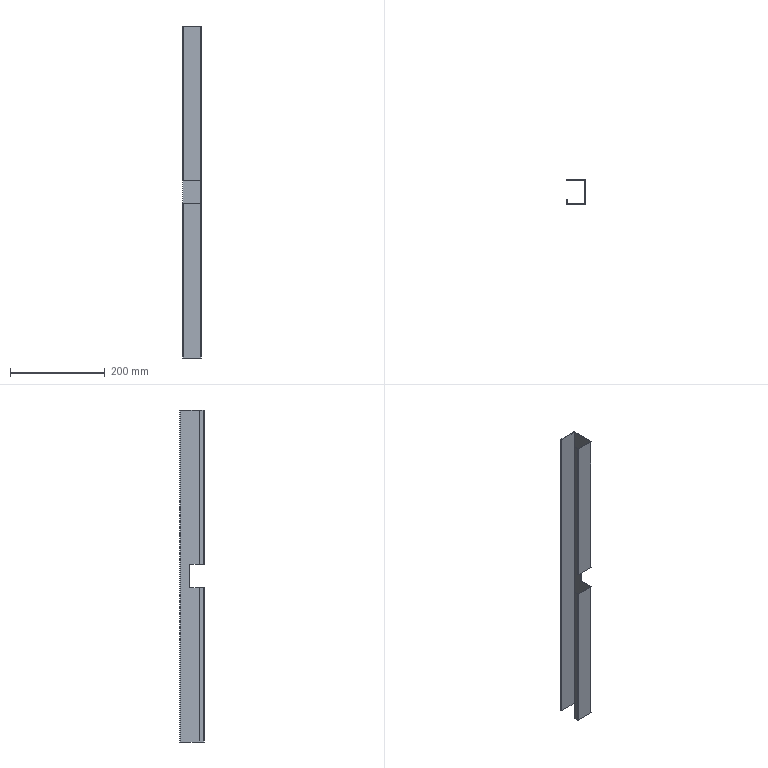Part | SolidWorks | features FlatPattern 1, ICE 1, SMBaseFlange 1, SheetMetal 1 | 1 solid | 50 faces | box 40 x 51 x 700 mm | volume 136327 mm3 | plane 40 | cylinder 10 | commonest cylinder face diameters 0.4 x5 3.4 x5
STEP:
#1=CARTESIAN_POINT('',(-20.,-41.,-25.));
#2=VERTEX_POINT('',#1);
#3=CARTESIAN_POINT('',(-20.,-49.3,-25.));
#4=VERTEX_POINT('',#3);
#5=CARTESIAN_POINT('',(-20.,-51.,-25.));
#6=DIRECTION('',(0.,-1.,0.));
#7=VECTOR('',#6,1000.);
#8=LINE('',#5,#7);
#9=EDGE_CURVE('',#2,#4,#8,.T.);
#10=ORIENTED_EDGE('',*,*,#9,.T.);
#11=CARTESIAN_POINT('',(-18.5,-49.3,-25.));
#12=VERTEX_POINT('',#11);
#13=CARTESIAN_POINT('',(-20.,-49.3,-25.));
#14=DIRECTION('',(1.,0.,0.));
#15=VECTOR('',#14,1000.);
#16=LINE('',#13,#15);
#17=EDGE_CURVE('',#4,#12,#16,.T.);
#18=ORIENTED_EDGE('',*,*,#17,.T.);
#19=CARTESIAN_POINT('',(-18.5,-41.,-25.));
#20=VERTEX_POINT('',#19);
#21=CARTESIAN_POINT('',(-18.5,-51.,-25.));
#22=DIRECTION('',(0.,-1.,0.));
#23=VECTOR('',#22,1000.);
#24=LINE('',#21,#23);
#25=EDGE_CURVE('',#20,#12,#24,.T.);
#26=ORIENTED_EDGE('',*,*,#25,.F.);
#27=CARTESIAN_POINT('',(-20.,-41.,-25.));
#28=DIRECTION('',(-1.,0.,0.));
#29=VECTOR('',#28,1000.);
#30=LINE('',#27,#29);
#31=EDGE_CURVE('',#20,#2,#30,.T.);
#32=ORIENTED_EDGE('',*,*,#31,.T.);
#33=EDGE_LOOP('',(#10,#18,#26,#32));
#34=FACE_OUTER_BOUND('',#33,.T.);
#35=CARTESIAN_POINT('',(40.,-21.,-25.));
#36=DIRECTION('',(0.,0.,-1.));
#37=DIRECTION('',(-1.,0.,0.));
#38=AXIS2_PLACEMENT_3D('',#35,#36,#37);
#39=PLANE('',#38);
#40=ADVANCED_FACE('',(#34),#39,.F.);
#41=CARTESIAN_POINT('',(-18.3,-49.5,-25.));
#42=VERTEX_POINT('',#41);
#43=CARTESIAN_POINT('',(18.3,-49.5,-25.));
#44=VERTEX_POINT('',#43);
#45=CARTESIAN_POINT('',(20.,-49.5,-25.));
#46=DIRECTION('',(1.,0.,0.));
#47=VECTOR('',#46,1000.);
#48=LINE('',#45,#47);
#49=EDGE_CURVE('',#42,#44,#48,.T.);
#50=ORIENTED_EDGE('',*,*,#49,.F.);
#51=CARTESIAN_POINT('',(-18.3,-51.,-25.));
#52=VERTEX_POINT('',#51);
#53=CARTESIAN_POINT('',(-18.3,-49.5,-25.));
#54=DIRECTION('',(0.,-1.,0.));
#55=VECTOR('',#54,1000.);
#56=LINE('',#53,#55);
#57=EDGE_CURVE('',#42,#52,#56,.T.);
#58=ORIENTED_EDGE('',*,*,#57,.T.);
#59=CARTESIAN_POINT('',(18.3,-51.,-25.));
#60=VERTEX_POINT('',#59);
#61=CARTESIAN_POINT('',(40.,-51.,-25.));
#62=DIRECTION('',(1.,0.,0.));
#63=VECTOR('',#62,1000.);
#64=LINE('',#61,#63);
#65=EDGE_CURVE('',#52,#60,#64,.T.);
#66=ORIENTED_EDGE('',*,*,#65,.T.);
#67=CARTESIAN_POINT('',(18.3,-51.,-25.));
#68=DIRECTION('',(0.,1.,0.));
#69=VECTOR('',#68,1000.);
#70=LINE('',#67,#69);
#71=EDGE_CURVE('',#60,#44,#70,.T.);
#72=ORIENTED_EDGE('',*,*,#71,.T.);
#73=EDGE_LOOP('',(#50,#58,#66,#72));
#74=FACE_OUTER_BOUND('',#73,.T.);
#75=CARTESIAN_POINT('',(40.,-21.,-25.));
#76=DIRECTION('',(0.,0.,-1.));
#77=DIRECTION('',(-1.,0.,0.));
#78=AXIS2_PLACEMENT_3D('',#75,#76,#77);
#79=PLANE('',#78);
#80=ADVANCED_FACE('',(#74),#79,.F.);
#81=CARTESIAN_POINT('',(18.5,-49.3,-25.));
#82=VERTEX_POINT('',#81);
#83=CARTESIAN_POINT('',(18.5,-21.,-25.));
#84=VERTEX_POINT('',#83);
#85=CARTESIAN_POINT('',(18.5,0.,-25.));
#86=DIRECTION('',(0.,1.,0.));
#87=VECTOR('',#86,1000.);
#88=LINE('',#85,#87);
#89=EDGE_CURVE('',#82,#84,#88,.T.);
#90=ORIENTED_EDGE('',*,*,#89,.F.);
#91=CARTESIAN_POINT('',(20.,-49.3,-25.));
#92=VERTEX_POINT('',#91);
#93=CARTESIAN_POINT('',(18.5,-49.3,-25.));
#94=DIRECTION('',(1.,0.,0.));
#95=VECTOR('',#94,1000.);
#96=LINE('',#93,#95);
#97=EDGE_CURVE('',#82,#92,#96,.T.);
#98=ORIENTED_EDGE('',*,*,#97,.T.);
#99=CARTESIAN_POINT('',(20.,-21.,-25.));
#100=VERTEX_POINT('',#99);
#101=CARTESIAN_POINT('',(20.,0.,-25.));
#102=DIRECTION('',(0.,1.,0.));
#103=VECTOR('',#102,1000.);
#104=LINE('',#101,#103);
#105=EDGE_CURVE('',#92,#100,#104,.T.);
#106=ORIENTED_EDGE('',*,*,#105,.T.);
#107=CARTESIAN_POINT('',(40.,-21.,-25.));
#108=DIRECTION('',(1.,0.,0.));
#109=VECTOR('',#108,1000.);
#110=LINE('',#107,#109);
#111=EDGE_CURVE('',#84,#100,#110,.T.);
#112=ORIENTED_EDGE('',*,*,#111,.F.);
#113=EDGE_LOOP('',(#90,#98,#106,#112));
#114=FACE_OUTER_BOUND('',#113,.T.);
#115=CARTESIAN_POINT('',(40.,-21.,-25.));
#116=DIRECTION('',(0.,0.,-1.));
#117=DIRECTION('',(-1.,0.,0.));
#118=AXIS2_PLACEMENT_3D('',#115,#116,#117);
#119=PLANE('',#118);
#120=ADVANCED_FACE('',(#114),#119,.F.);
#121=ORIENTED_EDGE('',*,*,#17,.F.);
#122=CARTESIAN_POINT('',(-18.3,-49.3,-25.));
#123=DIRECTION('',(0.,0.,1.));
#124=DIRECTION('',(-1.,0.,0.));
#125=AXIS2_PLACEMENT_3D('',#122,#123,#124);
#126=CIRCLE('',#125,1.7);
#127=EDGE_CURVE('',#4,#52,#126,.T.);
#128=ORIENTED_EDGE('',*,*,#127,.T.);
#129=ORIENTED_EDGE('',*,*,#57,.F.);
#130=CARTESIAN_POINT('',(-18.3,-49.3,-25.));
#131=DIRECTION('',(0.,0.,1.));
#132=DIRECTION('',(-1.,0.,0.));
#133=AXIS2_PLACEMENT_3D('',#130,#131,#132);
#134=CIRCLE('',#133,0.2);
#135=EDGE_CURVE('',#12,#42,#134,.T.);
#136=ORIENTED_EDGE('',*,*,#135,.F.);
#137=EDGE_LOOP('',(#121,#128,#129,#136));
#138=FACE_OUTER_BOUND('',#137,.T.);
#139=CARTESIAN_POINT('',(40.,-21.,-25.));
#140=DIRECTION('',(0.,0.,-1.));
#141=DIRECTION('',(-1.,0.,0.));
#142=AXIS2_PLACEMENT_3D('',#139,#140,#141);
#143=PLANE('',#142);
#144=ADVANCED_FACE('',(#138),#143,.F.);
#145=CARTESIAN_POINT('',(-18.5,-49.3,25.));
#146=VERTEX_POINT('',#145);
#147=CARTESIAN_POINT('',(-18.5,-41.,25.));
#148=VERTEX_POINT('',#147);
#149=CARTESIAN_POINT('',(-18.5,-51.,25.));
#150=DIRECTION('',(0.,1.,0.));
#151=VECTOR('',#150,1000.);
#152=LINE('',#149,#151);
#153=EDGE_CURVE('',#146,#148,#152,.T.);
#154=ORIENTED_EDGE('',*,*,#153,.F.);
#155=CARTESIAN_POINT('',(-20.,-49.3,25.));
#156=VERTEX_POINT('',#155);
#157=CARTESIAN_POINT('',(-18.5,-49.3,25.));
#158=DIRECTION('',(-1.,0.,0.));
#159=VECTOR('',#158,1000.);
#160=LINE('',#157,#159);
#161=EDGE_CURVE('',#146,#156,#160,.T.);
#162=ORIENTED_EDGE('',*,*,#161,.T.);
#163=CARTESIAN_POINT('',(-20.,-41.,25.));
#164=VERTEX_POINT('',#163);
#165=CARTESIAN_POINT('',(-20.,-51.,25.));
#166=DIRECTION('',(0.,1.,0.));
#167=VECTOR('',#166,1000.);
#168=LINE('',#165,#167);
#169=EDGE_CURVE('',#156,#164,#168,.T.);
#170=ORIENTED_EDGE('',*,*,#169,.T.);
#171=CARTESIAN_POINT('',(-20.,-41.,25.));
#172=DIRECTION('',(1.,0.,0.));
#173=VECTOR('',#172,1000.);
#174=LINE('',#171,#173);
#175=EDGE_CURVE('',#164,#148,#174,.T.);
#176=ORIENTED_EDGE('',*,*,#175,.T.);
#177=EDGE_LOOP('',(#154,#162,#170,#176));
#178=FACE_OUTER_BOUND('',#177,.T.);
#179=CARTESIAN_POINT('',(40.,-21.,25.));
#180=DIRECTION('',(0.,0.,1.));
#181=DIRECTION('',(1.,0.,0.));
#182=AXIS2_PLACEMENT_3D('',#179,#180,#181);
#183=PLANE('',#182);
#184=ADVANCED_FACE('',(#178),#183,.F.);
#185=CARTESIAN_POINT('',(18.3,-51.,25.));
#186=VERTEX_POINT('',#185);
#187=CARTESIAN_POINT('',(-18.3,-51.,25.));
#188=VERTEX_POINT('',#187);
#189=CARTESIAN_POINT('',(40.,-51.,25.));
#190=DIRECTION('',(-1.,0.,0.));
#191=VECTOR('',#190,1000.);
#192=LINE('',#189,#191);
#193=EDGE_CURVE('',#186,#188,#192,.T.);
#194=ORIENTED_EDGE('',*,*,#193,.T.);
#195=CARTESIAN_POINT('',(-18.3,-49.5,25.));
#196=VERTEX_POINT('',#195);
#197=CARTESIAN_POINT('',(-18.3,-51.,25.));
#198=DIRECTION('',(0.,1.,0.));
#199=VECTOR('',#198,1000.);
#200=LINE('',#197,#199);
#201=EDGE_CURVE('',#188,#196,#200,.T.);
#202=ORIENTED_EDGE('',*,*,#201,.T.);
#203=CARTESIAN_POINT('',(18.3,-49.5,25.));
#204=VERTEX_POINT('',#203);
#205=CARTESIAN_POINT('',(20.,-49.5,25.));
#206=DIRECTION('',(-1.,0.,0.));
#207=VECTOR('',#206,1000.);
#208=LINE('',#205,#207);
#209=EDGE_CURVE('',#204,#196,#208,.T.);
#210=ORIENTED_EDGE('',*,*,#209,.F.);
#211=CARTESIAN_POINT('',(18.3,-49.5,25.));
#212=DIRECTION('',(0.,-1.,0.));
#213=VECTOR('',#212,1000.);
#214=LINE('',#211,#213);
#215=EDGE_CURVE('',#204,#186,#214,.T.);
#216=ORIENTED_EDGE('',*,*,#215,.T.);
#217=EDGE_LOOP('',(#194,#202,#210,#216));
#218=FACE_OUTER_BOUND('',#217,.T.);
#219=CARTESIAN_POINT('',(40.,-21.,25.));
#220=DIRECTION('',(0.,0.,1.));
#221=DIRECTION('',(1.,0.,0.));
#222=AXIS2_PLACEMENT_3D('',#219,#220,#221);
#223=PLANE('',#222);
#224=ADVANCED_FACE('',(#218),#223,.F.);
#225=ORIENTED_EDGE('',*,*,#161,.F.);
#226=CARTESIAN_POINT('',(-18.3,-49.3,25.));
#227=DIRECTION('',(0.,0.,-1.));
#228=DIRECTION('',(1.,0.,0.));
#229=AXIS2_PLACEMENT_3D('',#226,#227,#228);
#230=CIRCLE('',#229,0.2);
#231=EDGE_CURVE('',#196,#146,#230,.T.);
#232=ORIENTED_EDGE('',*,*,#231,.F.);
#233=ORIENTED_EDGE('',*,*,#201,.F.);
#234=CARTESIAN_POINT('',(-18.3,-49.3,25.));
#235=DIRECTION('',(0.,0.,-1.));
#236=DIRECTION('',(1.,0.,0.));
#237=AXIS2_PLACEMENT_3D('',#234,#235,#236);
#238=CIRCLE('',#237,1.7);
#239=EDGE_CURVE('',#188,#156,#238,.T.);
#240=ORIENTED_EDGE('',*,*,#239,.T.);
#241=EDGE_LOOP('',(#225,#232,#233,#240));
#242=FACE_OUTER_BOUND('',#241,.T.);
#243=CARTESIAN_POINT('',(40.,-21.,25.));
#244=DIRECTION('',(0.,0.,1.));
#245=DIRECTION('',(1.,0.,0.));
#246=AXIS2_PLACEMENT_3D('',#243,#244,#245);
#247=PLANE('',#246);
#248=ADVANCED_FACE('',(#242),#247,.F.);
#249=CARTESIAN_POINT('',(20.,-21.,25.));
#250=VERTEX_POINT('',#249);
#251=CARTESIAN_POINT('',(20.,-49.3,25.));
#252=VERTEX_POINT('',#251);
#253=CARTESIAN_POINT('',(20.,0.,25.));
#254=DIRECTION('',(0.,-1.,0.));
#255=VECTOR('',#254,1000.);
#256=LINE('',#253,#255);
#257=EDGE_CURVE('',#250,#252,#256,.T.);
#258=ORIENTED_EDGE('',*,*,#257,.T.);
#259=CARTESIAN_POINT('',(18.5,-49.3,25.));
#260=VERTEX_POINT('',#259);
#261=CARTESIAN_POINT('',(20.,-49.3,25.));
#262=DIRECTION('',(-1.,0.,0.));
#263=VECTOR('',#262,1000.);
#264=LINE('',#261,#263);
#265=EDGE_CURVE('',#252,#260,#264,.T.);
#266=ORIENTED_EDGE('',*,*,#265,.T.);
#267=CARTESIAN_POINT('',(18.5,-21.,25.));
#268=VERTEX_POINT('',#267);
#269=CARTESIAN_POINT('',(18.5,0.,25.));
#270=DIRECTION('',(0.,-1.,0.));
#271=VECTOR('',#270,1000.);
#272=LINE('',#269,#271);
#273=EDGE_CURVE('',#268,#260,#272,.T.);
#274=ORIENTED_EDGE('',*,*,#273,.F.);
#275=CARTESIAN_POINT('',(40.,-21.,25.));
#276=DIRECTION('',(-1.,0.,0.));
#277=VECTOR('',#276,1000.);
#278=LINE('',#275,#277);
#279=EDGE_CURVE('',#250,#268,#278,.T.);
#280=ORIENTED_EDGE('',*,*,#279,.F.);
#281=EDGE_LOOP('',(#258,#266,#274,#280));
#282=FACE_OUTER_BOUND('',#281,.T.);
#283=CARTESIAN_POINT('',(40.,-21.,25.));
#284=DIRECTION('',(0.,0.,1.));
#285=DIRECTION('',(1.,0.,0.));
#286=AXIS2_PLACEMENT_3D('',#283,#284,#285);
#287=PLANE('',#286);
#288=ADVANCED_FACE('',(#282),#287,.F.);
#289=CARTESIAN_POINT('',(-18.5,-49.3,350.));
#290=VERTEX_POINT('',#289);
#291=CARTESIAN_POINT('',(-18.5,-49.3,350.));
#292=DIRECTION('',(0.,0.,-1.));
#293=VECTOR('',#292,1000.);
#294=LINE('',#291,#293);
#295=EDGE_CURVE('',#290,#146,#294,.T.);
#296=ORIENTED_EDGE('',*,*,#295,.T.);
#297=ORIENTED_EDGE('',*,*,#153,.T.);
#298=CARTESIAN_POINT('',(-18.5,-41.,350.));
#299=VERTEX_POINT('',#298);
#300=CARTESIAN_POINT('',(-18.5,-41.,350.));
#301=DIRECTION('',(0.,0.,-1.));
#302=VECTOR('',#301,1000.);
#303=LINE('',#300,#302);
#304=EDGE_CURVE('',#299,#148,#303,.T.);
#305=ORIENTED_EDGE('',*,*,#304,.F.);
#306=CARTESIAN_POINT('',(-18.5,-51.,350.));
#307=DIRECTION('',(0.,1.,0.));
#308=VECTOR('',#307,1000.);
#309=LINE('',#306,#308);
#310=EDGE_CURVE('',#290,#299,#309,.T.);
#311=ORIENTED_EDGE('',*,*,#310,.F.);
#312=EDGE_LOOP('',(#296,#297,#305,#311));
#313=FACE_OUTER_BOUND('',#312,.T.);
#314=CARTESIAN_POINT('',(-18.5,-51.,350.));
#315=DIRECTION('',(-1.,0.,0.));
#316=DIRECTION('',(0.,-1.,0.));
#317=AXIS2_PLACEMENT_3D('',#314,#315,#316);
#318=PLANE('',#317);
#319=ADVANCED_FACE('',(#313),#318,.F.);
#320=ORIENTED_EDGE('',*,*,#175,.F.);
#321=CARTESIAN_POINT('',(-20.,-41.,350.));
#322=VERTEX_POINT('',#321);
#323=CARTESIAN_POINT('',(-20.,-41.,350.));
#324=DIRECTION('',(0.,0.,-1.));
#325=VECTOR('',#324,1000.);
#326=LINE('',#323,#325);
#327=EDGE_CURVE('',#322,#164,#326,.T.);
#328=ORIENTED_EDGE('',*,*,#327,.F.);
#329=CARTESIAN_POINT('',(-20.,-41.,350.));
#330=DIRECTION('',(1.,0.,0.));
#331=VECTOR('',#330,1000.);
#332=LINE('',#329,#331);
#333=EDGE_CURVE('',#322,#299,#332,.T.);
#334=ORIENTED_EDGE('',*,*,#333,.T.);
#335=ORIENTED_EDGE('',*,*,#304,.T.);
#336=EDGE_LOOP('',(#320,#328,#334,#335));
#337=FACE_OUTER_BOUND('',#336,.T.);
#338=CARTESIAN_POINT('',(-20.,-41.,350.));
#339=DIRECTION('',(0.,1.,0.));
#340=DIRECTION('',(0.,0.,1.));
#341=AXIS2_PLACEMENT_3D('',#338,#339,#340);
#342=PLANE('',#341);
#343=ADVANCED_FACE('',(#337),#342,.T.);
#344=ORIENTED_EDGE('',*,*,#169,.F.);
#345=CARTESIAN_POINT('',(-20.,-49.3,350.));
#346=VERTEX_POINT('',#345);
#347=CARTESIAN_POINT('',(-20.,-49.3,350.));
#348=DIRECTION('',(0.,0.,-1.));
#349=VECTOR('',#348,1000.);
#350=LINE('',#347,#349);
#351=EDGE_CURVE('',#346,#156,#350,.T.);
#352=ORIENTED_EDGE('',*,*,#351,.F.);
#353=CARTESIAN_POINT('',(-20.,-51.,350.));
#354=DIRECTION('',(0.,1.,0.));
#355=VECTOR('',#354,1000.);
#356=LINE('',#353,#355);
#357=EDGE_CURVE('',#346,#322,#356,.T.);
#358=ORIENTED_EDGE('',*,*,#357,.T.);
#359=ORIENTED_EDGE('',*,*,#327,.T.);
#360=EDGE_LOOP('',(#344,#352,#358,#359));
#361=FACE_OUTER_BOUND('',#360,.T.);
#362=CARTESIAN_POINT('',(-20.,-51.,350.));
#363=DIRECTION('',(-1.,0.,0.));
#364=DIRECTION('',(0.,-1.,0.));
#365=AXIS2_PLACEMENT_3D('',#362,#363,#364);
#366=PLANE('',#365);
#367=ADVANCED_FACE('',(#361),#366,.T.);
#368=ORIENTED_EDGE('',*,*,#239,.F.);
#369=CARTESIAN_POINT('',(-18.3,-51.,350.));
#370=VERTEX_POINT('',#369);
#371=CARTESIAN_POINT('',(-18.3,-51.,350.));
#372=DIRECTION('',(0.,0.,-1.));
#373=VECTOR('',#372,1000.);
#374=LINE('',#371,#373);
#375=EDGE_CURVE('',#370,#188,#374,.T.);
#376=ORIENTED_EDGE('',*,*,#375,.F.);
#377=CARTESIAN_POINT('',(-18.3,-49.3,350.));
#378=DIRECTION('',(0.,0.,-1.));
#379=DIRECTION('',(1.,0.,0.));
#380=AXIS2_PLACEMENT_3D('',#377,#378,#379);
#381=CIRCLE('',#380,1.7);
#382=EDGE_CURVE('',#370,#346,#381,.T.);
#383=ORIENTED_EDGE('',*,*,#382,.T.);
#384=ORIENTED_EDGE('',*,*,#351,.T.);
#385=EDGE_LOOP('',(#368,#376,#383,#384));
#386=FACE_OUTER_BOUND('',#385,.T.);
#387=CARTESIAN_POINT('',(-18.3,-49.3,350.));
#388=DIRECTION('',(0.,0.,-1.));
#389=DIRECTION('',(-1.,0.,0.));
#390=AXIS2_PLACEMENT_3D('',#387,#388,#389);
#391=CYLINDRICAL_SURFACE('',#390,1.7);
#392=ADVANCED_FACE('',(#386),#391,.T.);
#393=ORIENTED_EDGE('',*,*,#193,.F.);
#394=CARTESIAN_POINT('',(18.3,-51.,350.));
#395=VERTEX_POINT('',#394);
#396=CARTESIAN_POINT('',(18.3,-51.,350.));
#397=DIRECTION('',(0.,0.,-1.));
#398=VECTOR('',#397,1000.);
#399=LINE('',#396,#398);
#400=EDGE_CURVE('',#395,#186,#399,.T.);
#401=ORIENTED_EDGE('',*,*,#400,.F.);
#402=CARTESIAN_POINT('',(20.,-51.,350.));
#403=DIRECTION('',(-1.,0.,0.));
#404=VECTOR('',#403,1000.);
#405=LINE('',#402,#404);
#406=EDGE_CURVE('',#395,#370,#405,.T.);
#407=ORIENTED_EDGE('',*,*,#406,.T.);
#408=ORIENTED_EDGE('',*,*,#375,.T.);
#409=EDGE_LOOP('',(#393,#401,#407,#408));
#410=FACE_OUTER_BOUND('',#409,.T.);
#411=CARTESIAN_POINT('',(20.,-51.,350.));
#412=DIRECTION('',(0.,-1.,0.));
#413=DIRECTION('',(1.,0.,0.));
#414=AXIS2_PLACEMENT_3D('',#411,#412,#413);
#415=PLANE('',#414);
#416=ADVANCED_FACE('',(#410),#415,.T.);
#417=CARTESIAN_POINT('',(18.3,-49.3,25.));
#418=DIRECTION('',(0.,0.,-1.));
#419=DIRECTION('',(1.,0.,0.));
#420=AXIS2_PLACEMENT_3D('',#417,#418,#419);
#421=CIRCLE('',#420,1.7);
#422=EDGE_CURVE('',#252,#186,#421,.T.);
#423=ORIENTED_EDGE('',*,*,#422,.F.);
#424=CARTESIAN_POINT('',(20.,-49.3,350.));
#425=VERTEX_POINT('',#424);
#426=CARTESIAN_POINT('',(20.,-49.3,350.));
#427=DIRECTION('',(0.,0.,-1.));
#428=VECTOR('',#427,1000.);
#429=LINE('',#426,#428);
#430=EDGE_CURVE('',#425,#252,#429,.T.);
#431=ORIENTED_EDGE('',*,*,#430,.F.);
#432=CARTESIAN_POINT('',(18.3,-49.3,350.));
#433=DIRECTION('',(0.,0.,-1.));
#434=DIRECTION('',(1.,0.,0.));
#435=AXIS2_PLACEMENT_3D('',#432,#433,#434);
#436=CIRCLE('',#435,1.7);
#437=EDGE_CURVE('',#425,#395,#436,.T.);
#438=ORIENTED_EDGE('',*,*,#437,.T.);
#439=ORIENTED_EDGE('',*,*,#400,.T.);
#440=EDGE_LOOP('',(#423,#431,#438,#439));
#441=FACE_OUTER_BOUND('',#440,.T.);
#442=CARTESIAN_POINT('',(18.3,-49.3,350.));
#443=DIRECTION('',(0.,0.,-1.));
#444=DIRECTION('',(-1.,0.,0.));
#445=AXIS2_PLACEMENT_3D('',#442,#443,#444);
#446=CYLINDRICAL_SURFACE('',#445,1.7);
#447=ADVANCED_FACE('',(#441),#446,.T.);
#448=CARTESIAN_POINT('',(18.5,-49.3,350.));
#449=VERTEX_POINT('',#448);
#450=CARTESIAN_POINT('',(18.5,-49.3,350.));
#451=DIRECTION('',(0.,0.,-1.));
#452=VECTOR('',#451,1000.);
#453=LINE('',#450,#452);
#454=EDGE_CURVE('',#449,#260,#453,.T.);
#455=ORIENTED_EDGE('',*,*,#454,.T.);
#456=CARTESIAN_POINT('',(18.3,-49.3,25.));
#457=DIRECTION('',(0.,0.,-1.));
#458=DIRECTION('',(1.,0.,0.));
#459=AXIS2_PLACEMENT_3D('',#456,#457,#458);
#460=CIRCLE('',#459,0.2);
#461=EDGE_CURVE('',#260,#204,#460,.T.);
#462=ORIENTED_EDGE('',*,*,#461,.T.);
#463=CARTESIAN_POINT('',(18.3,-49.5,350.));
#464=VERTEX_POINT('',#463);
#465=CARTESIAN_POINT('',(18.3,-49.5,350.));
#466=DIRECTION('',(0.,0.,-1.));
#467=VECTOR('',#466,1000.);
#468=LINE('',#465,#467);
#469=EDGE_CURVE('',#464,#204,#468,.T.);
#470=ORIENTED_EDGE('',*,*,#469,.F.);
#471=CARTESIAN_POINT('',(18.3,-49.3,350.));
#472=DIRECTION('',(0.,0.,-1.));
#473=DIRECTION('',(1.,0.,0.));
#474=AXIS2_PLACEMENT_3D('',#471,#472,#473);
#475=CIRCLE('',#474,0.2);
#476=EDGE_CURVE('',#449,#464,#475,.T.);
#477=ORIENTED_EDGE('',*,*,#476,.F.);
#478=EDGE_LOOP('',(#455,#462,#470,#477));
#479=FACE_OUTER_BOUND('',#478,.T.);
#480=CARTESIAN_POINT('',(18.3,-49.3,350.));
#481=DIRECTION('',(0.,0.,-1.));
#482=DIRECTION('',(-1.,0.,0.));
#483=AXIS2_PLACEMENT_3D('',#480,#481,#482);
#484=CYLINDRICAL_SURFACE('',#483,0.2);
#485=ADVANCED_FACE('',(#479),#484,.F.);
#486=ORIENTED_EDGE('',*,*,#469,.T.);
#487=ORIENTED_EDGE('',*,*,#209,.T.);
#488=CARTESIAN_POINT('',(-18.3,-49.5,350.));
#489=VERTEX_POINT('',#488);
#490=CARTESIAN_POINT('',(-18.3,-49.5,350.));
#491=DIRECTION('',(0.,0.,-1.));
#492=VECTOR('',#491,1000.);
#493=LINE('',#490,#492);
#494=EDGE_CURVE('',#489,#196,#493,.T.);
#495=ORIENTED_EDGE('',*,*,#494,.F.);
#496=CARTESIAN_POINT('',(20.,-49.5,350.));
#497=DIRECTION('',(-1.,0.,0.));
#498=VECTOR('',#497,1000.);
#499=LINE('',#496,#498);
#500=EDGE_CURVE('',#464,#489,#499,.T.);
#501=ORIENTED_EDGE('',*,*,#500,.F.);
#502=EDGE_LOOP('',(#486,#487,#495,#501));
#503=FACE_OUTER_BOUND('',#502,.T.);
#504=CARTESIAN_POINT('',(20.,-49.5,350.));
#505=DIRECTION('',(0.,-1.,0.));
#506=DIRECTION('',(1.,0.,0.));
#507=AXIS2_PLACEMENT_3D('',#504,#505,#506);
#508=PLANE('',#507);
#509=ADVANCED_FACE('',(#503),#508,.F.);
#510=ORIENTED_EDGE('',*,*,#494,.T.);
#511=ORIENTED_EDGE('',*,*,#231,.T.);
#512=ORIENTED_EDGE('',*,*,#295,.F.);
#513=CARTESIAN_POINT('',(-18.3,-49.3,350.));
#514=DIRECTION('',(0.,0.,-1.));
#515=DIRECTION('',(1.,0.,0.));
#516=AXIS2_PLACEMENT_3D('',#513,#514,#515);
#517=CIRCLE('',#516,0.2);
#518=EDGE_CURVE('',#489,#290,#517,.T.);
#519=ORIENTED_EDGE('',*,*,#518,.F.);
#520=EDGE_LOOP('',(#510,#511,#512,#519));
#521=FACE_OUTER_BOUND('',#520,.T.);
#522=CARTESIAN_POINT('',(-18.3,-49.3,350.));
#523=DIRECTION('',(0.,0.,-1.));
#524=DIRECTION('',(-1.,0.,0.));
#525=AXIS2_PLACEMENT_3D('',#522,#523,#524);
#526=CYLINDRICAL_SURFACE('',#525,0.2);
#527=ADVANCED_FACE('',(#521),#526,.F.);
#528=CARTESIAN_POINT('',(20.,-1.7,350.));
#529=VERTEX_POINT('',#528);
#530=CARTESIAN_POINT('',(18.5,-1.7,350.));
#531=VERTEX_POINT('',#530);
#532=CARTESIAN_POINT('',(20.,-1.7,350.));
#533=DIRECTION('',(-1.,0.,0.));
#534=VECTOR('',#533,1000.);
#535=LINE('',#532,#534);
#536=EDGE_CURVE('',#529,#531,#535,.T.);
#537=ORIENTED_EDGE('',*,*,#536,.F.);
#538=CARTESIAN_POINT('',(18.3,0.,350.));
#539=VERTEX_POINT('',#538);
#540=CARTESIAN_POINT('',(18.3,-1.7,350.));
#541=DIRECTION('',(0.,0.,-1.));
#542=DIRECTION('',(1.,0.,0.));
#543=AXIS2_PLACEMENT_3D('',#540,#541,#542);
#544=CIRCLE('',#543,1.7);
#545=EDGE_CURVE('',#539,#529,#544,.T.);
#546=ORIENTED_EDGE('',*,*,#545,.F.);
#547=CARTESIAN_POINT('',(18.3,-1.5,350.));
#548=VERTEX_POINT('',#547);
#549=CARTESIAN_POINT('',(18.3,-1.5,350.));
#550=DIRECTION('',(0.,1.,0.));
#551=VECTOR('',#550,1000.);
#552=LINE('',#549,#551);
#553=EDGE_CURVE('',#548,#539,#552,.T.);
#554=ORIENTED_EDGE('',*,*,#553,.F.);
#555=CARTESIAN_POINT('',(18.3,-1.7,350.));
#556=DIRECTION('',(0.,0.,-1.));
#557=DIRECTION('',(1.,0.,0.));
#558=AXIS2_PLACEMENT_3D('',#555,#556,#557);
#559=CIRCLE('',#558,0.2);
#560=EDGE_CURVE('',#548,#531,#559,.T.);
#561=ORIENTED_EDGE('',*,*,#560,.T.);
#562=EDGE_LOOP('',(#537,#546,#554,#561));
#563=FACE_OUTER_BOUND('',#562,.T.);
#564=CARTESIAN_POINT('',(20.,-1.7,350.));
#565=DIRECTION('',(0.,0.,1.));
#566=DIRECTION('',(1.,0.,0.));
#567=AXIS2_PLACEMENT_3D('',#564,#565,#566);
#568=PLANE('',#567);
#569=ADVANCED_FACE('',(#563),#568,.T.);
#570=CARTESIAN_POINT('',(20.,0.,350.));
#571=DIRECTION('',(0.,-1.,0.));
#572=VECTOR('',#571,1000.);
#573=LINE('',#570,#572);
#574=EDGE_CURVE('',#529,#425,#573,.T.);
#575=ORIENTED_EDGE('',*,*,#574,.F.);
#576=ORIENTED_EDGE('',*,*,#536,.T.);
#577=CARTESIAN_POINT('',(18.5,0.,350.));
#578=DIRECTION('',(0.,-1.,0.));
#579=VECTOR('',#578,1000.);
#580=LINE('',#577,#579);
#581=EDGE_CURVE('',#531,#449,#580,.T.);
#582=ORIENTED_EDGE('',*,*,#581,.T.);
#583=CARTESIAN_POINT('',(18.5,-49.3,350.));
#584=DIRECTION('',(1.,0.,0.));
#585=VECTOR('',#584,1000.);
#586=LINE('',#583,#585);
#587=EDGE_CURVE('',#449,#425,#586,.T.);
#588=ORIENTED_EDGE('',*,*,#587,.T.);
#589=EDGE_LOOP('',(#575,#576,#582,#588));
#590=FACE_OUTER_BOUND('',#589,.T.);
#591=CARTESIAN_POINT('',(18.3,-1.5,350.));
#592=DIRECTION('',(0.,0.,1.));
#593=DIRECTION('',(1.,0.,0.));
#594=AXIS2_PLACEMENT_3D('',#591,#592,#593);
#595=PLANE('',#594);
#596=ADVANCED_FACE('',(#590),#595,.T.);
#597=CARTESIAN_POINT('',(18.3,0.,-350.));
#598=VERTEX_POINT('',#597);
#599=CARTESIAN_POINT('',(18.3,-1.5,-350.));
#600=VERTEX_POINT('',#599);
#601=CARTESIAN_POINT('',(18.3,0.,-350.));
#602=DIRECTION('',(0.,-1.,0.));
#603=VECTOR('',#602,1000.);
#604=LINE('',#601,#603);
#605=EDGE_CURVE('',#598,#600,#604,.T.);
#606=ORIENTED_EDGE('',*,*,#605,.F.);
#607=CARTESIAN_POINT('',(20.,-1.7,-350.));
#608=VERTEX_POINT('',#607);
#609=CARTESIAN_POINT('',(18.3,-1.7,-350.));
#610=DIRECTION('',(0.,0.,-1.));
#611=DIRECTION('',(1.,0.,0.));
#612=AXIS2_PLACEMENT_3D('',#609,#610,#611);
#613=CIRCLE('',#612,1.7);
#614=EDGE_CURVE('',#598,#608,#613,.T.);
#615=ORIENTED_EDGE('',*,*,#614,.T.);
#616=CARTESIAN_POINT('',(18.5,-1.7,-350.));
#617=VERTEX_POINT('',#616);
#618=CARTESIAN_POINT('',(18.5,-1.7,-350.));
#619=DIRECTION('',(1.,0.,0.));
#620=VECTOR('',#619,1000.);
#621=LINE('',#618,#620);
#622=EDGE_CURVE('',#617,#608,#621,.T.);
#623=ORIENTED_EDGE('',*,*,#622,.F.);
#624=CARTESIAN_POINT('',(18.3,-1.7,-350.));
#625=DIRECTION('',(0.,0.,-1.));
#626=DIRECTION('',(1.,0.,0.));
#627=AXIS2_PLACEMENT_3D('',#624,#625,#626);
#628=CIRCLE('',#627,0.2);
#629=EDGE_CURVE('',#600,#617,#628,.T.);
#630=ORIENTED_EDGE('',*,*,#629,.F.);
#631=EDGE_LOOP('',(#606,#615,#623,#630));
#632=FACE_OUTER_BOUND('',#631,.T.);
#633=CARTESIAN_POINT('',(18.3,0.,-350.));
#634=DIRECTION('',(0.,0.,-1.));
#635=DIRECTION('',(-1.,0.,0.));
#636=AXIS2_PLACEMENT_3D('',#633,#634,#635);
#637=PLANE('',#636);
#638=ADVANCED_FACE('',(#632),#637,.T.);
#639=CARTESIAN_POINT('',(-20.,0.,-350.));
#640=VERTEX_POINT('',#639);
#641=CARTESIAN_POINT('',(-20.,0.,-350.));
#642=DIRECTION('',(1.,0.,0.));
#643=VECTOR('',#642,1000.);
#644=LINE('',#641,#643);
#645=EDGE_CURVE('',#640,#598,#644,.T.);
#646=ORIENTED_EDGE('',*,*,#645,.T.);
#647=ORIENTED_EDGE('',*,*,#605,.T.);
#648=CARTESIAN_POINT('',(-20.,-1.5,-350.));
#649=VERTEX_POINT('',#648);
#650=CARTESIAN_POINT('',(-20.,-1.5,-350.));
#651=DIRECTION('',(1.,0.,0.));
#652=VECTOR('',#651,1000.);
#653=LINE('',#650,#652);
#654=EDGE_CURVE('',#649,#600,#653,.T.);
#655=ORIENTED_EDGE('',*,*,#654,.F.);
#656=CARTESIAN_POINT('',(-20.,-1.5,-350.));
#657=DIRECTION('',(0.,1.,0.));
#658=VECTOR('',#657,1000.);
#659=LINE('',#656,#658);
#660=EDGE_CURVE('',#649,#640,#659,.T.);
#661=ORIENTED_EDGE('',*,*,#660,.T.);
#662=EDGE_LOOP('',(#646,#647,#655,#661));
#663=FACE_OUTER_BOUND('',#662,.T.);
#664=CARTESIAN_POINT('',(18.5,-1.7,-350.));
#665=DIRECTION('',(0.,0.,-1.));
#666=DIRECTION('',(-1.,0.,0.));
#667=AXIS2_PLACEMENT_3D('',#664,#665,#666);
#668=PLANE('',#667);
#669=ADVANCED_FACE('',(#663),#668,.T.);
#670=CARTESIAN_POINT('',(18.3,-51.,350.));
#671=DIRECTION('',(0.,1.,0.));
#672=VECTOR('',#671,1000.);
#673=LINE('',#670,#672);
#674=EDGE_CURVE('',#395,#464,#673,.T.);
#675=ORIENTED_EDGE('',*,*,#674,.F.);
#676=ORIENTED_EDGE('',*,*,#437,.F.);
#677=ORIENTED_EDGE('',*,*,#587,.F.);
#678=ORIENTED_EDGE('',*,*,#476,.T.);
#679=EDGE_LOOP('',(#675,#676,#677,#678));
#680=FACE_OUTER_BOUND('',#679,.T.);
#681=CARTESIAN_POINT('',(18.3,-51.,350.));
#682=DIRECTION('',(0.,0.,1.));
#683=DIRECTION('',(1.,0.,0.));
#684=AXIS2_PLACEMENT_3D('',#681,#682,#683);
#685=PLANE('',#684);
#686=ADVANCED_FACE('',(#680),#685,.T.);
#687=ORIENTED_EDGE('',*,*,#406,.F.);
#688=ORIENTED_EDGE('',*,*,#674,.T.);
#689=ORIENTED_EDGE('',*,*,#500,.T.);
#690=CARTESIAN_POINT('',(-18.3,-49.5,350.));
#691=DIRECTION('',(0.,-1.,0.));
#692=VECTOR('',#691,1000.);
#693=LINE('',#690,#692);
#694=EDGE_CURVE('',#489,#370,#693,.T.);
#695=ORIENTED_EDGE('',*,*,#694,.T.);
#696=EDGE_LOOP('',(#687,#688,#689,#695));
#697=FACE_OUTER_BOUND('',#696,.T.);
#698=CARTESIAN_POINT('',(18.5,-49.3,350.));
#699=DIRECTION('',(0.,0.,1.));
#700=DIRECTION('',(1.,0.,0.));
#701=AXIS2_PLACEMENT_3D('',#698,#699,#700);
#702=PLANE('',#701);
#703=ADVANCED_FACE('',(#697),#702,.T.);
#704=CARTESIAN_POINT('',(20.,-49.3,-350.));
#705=VERTEX_POINT('',#704);
#706=CARTESIAN_POINT('',(18.5,-49.3,-350.));
#707=VERTEX_POINT('',#706);
#708=CARTESIAN_POINT('',(20.,-49.3,-350.));
#709=DIRECTION('',(-1.,0.,0.));
#710=VECTOR('',#709,1000.);
#711=LINE('',#708,#710);
#712=EDGE_CURVE('',#705,#707,#711,.T.);
#713=ORIENTED_EDGE('',*,*,#712,.F.);
#714=CARTESIAN_POINT('',(18.3,-51.,-350.));
#715=VERTEX_POINT('',#714);
#716=CARTESIAN_POINT('',(18.3,-49.3,-350.));
#717=DIRECTION('',(0.,0.,-1.));
#718=DIRECTION('',(1.,0.,0.));
#719=AXIS2_PLACEMENT_3D('',#716,#717,#718);
#720=CIRCLE('',#719,1.7);
#721=EDGE_CURVE('',#705,#715,#720,.T.);
#722=ORIENTED_EDGE('',*,*,#721,.T.);
#723=CARTESIAN_POINT('',(18.3,-49.5,-350.));
#724=VERTEX_POINT('',#723);
#725=CARTESIAN_POINT('',(18.3,-49.5,-350.));
#726=DIRECTION('',(0.,-1.,0.));
#727=VECTOR('',#726,1000.);
#728=LINE('',#725,#727);
#729=EDGE_CURVE('',#724,#715,#728,.T.);
#730=ORIENTED_EDGE('',*,*,#729,.F.);
#731=CARTESIAN_POINT('',(18.3,-49.3,-350.));
#732=DIRECTION('',(0.,0.,-1.));
#733=DIRECTION('',(1.,0.,0.));
#734=AXIS2_PLACEMENT_3D('',#731,#732,#733);
#735=CIRCLE('',#734,0.2);
#736=EDGE_CURVE('',#707,#724,#735,.T.);
#737=ORIENTED_EDGE('',*,*,#736,.F.);
#738=EDGE_LOOP('',(#713,#722,#730,#737));
#739=FACE_OUTER_BOUND('',#738,.T.);
#740=CARTESIAN_POINT('',(20.,-49.3,-350.));
#741=DIRECTION('',(0.,0.,-1.));
#742=DIRECTION('',(-1.,0.,0.));
#743=AXIS2_PLACEMENT_3D('',#740,#741,#742);
#744=PLANE('',#743);
#745=ADVANCED_FACE('',(#739),#744,.T.);
#746=CARTESIAN_POINT('',(20.,0.,-350.));
#747=DIRECTION('',(0.,-1.,0.));
#748=VECTOR('',#747,1000.);
#749=LINE('',#746,#748);
#750=EDGE_CURVE('',#608,#705,#749,.T.);
#751=ORIENTED_EDGE('',*,*,#750,.T.);
#752=ORIENTED_EDGE('',*,*,#712,.T.);
#753=CARTESIAN_POINT('',(18.5,0.,-350.));
#754=DIRECTION('',(0.,-1.,0.));
#755=VECTOR('',#754,1000.);
#756=LINE('',#753,#755);
#757=EDGE_CURVE('',#617,#707,#756,.T.);
#758=ORIENTED_EDGE('',*,*,#757,.F.);
#759=ORIENTED_EDGE('',*,*,#622,.T.);
#760=EDGE_LOOP('',(#751,#752,#758,#759));
#761=FACE_OUTER_BOUND('',#760,.T.);
#762=CARTESIAN_POINT('',(18.3,-49.5,-350.));
#763=DIRECTION('',(0.,0.,-1.));
#764=DIRECTION('',(-1.,0.,0.));
#765=AXIS2_PLACEMENT_3D('',#762,#763,#764);
#766=PLANE('',#765);
#767=ADVANCED_FACE('',(#761),#766,.T.);
#768=CARTESIAN_POINT('',(-20.,-49.3,350.));
#769=DIRECTION('',(1.,0.,0.));
#770=VECTOR('',#769,1000.);
#771=LINE('',#768,#770);
#772=EDGE_CURVE('',#346,#290,#771,.T.);
#773=ORIENTED_EDGE('',*,*,#772,.F.);
#774=ORIENTED_EDGE('',*,*,#382,.F.);
#775=ORIENTED_EDGE('',*,*,#694,.F.);
#776=ORIENTED_EDGE('',*,*,#518,.T.);
#777=EDGE_LOOP('',(#773,#774,#775,#776));
#778=FACE_OUTER_BOUND('',#777,.T.);
#779=CARTESIAN_POINT('',(-20.,-49.3,350.));
#780=DIRECTION('',(0.,0.,1.));
#781=DIRECTION('',(1.,0.,0.));
#782=AXIS2_PLACEMENT_3D('',#779,#780,#781);
#783=PLANE('',#782);
#784=ADVANCED_FACE('',(#778),#783,.T.);
#785=ORIENTED_EDGE('',*,*,#357,.F.);
#786=ORIENTED_EDGE('',*,*,#772,.T.);
#787=ORIENTED_EDGE('',*,*,#310,.T.);
#788=ORIENTED_EDGE('',*,*,#333,.F.);
#789=EDGE_LOOP('',(#785,#786,#787,#788));
#790=FACE_OUTER_BOUND('',#789,.T.);
#791=CARTESIAN_POINT('',(-18.3,-49.5,350.));
#792=DIRECTION('',(0.,0.,1.));
#793=DIRECTION('',(1.,0.,0.));
#794=AXIS2_PLACEMENT_3D('',#791,#792,#793);
#795=PLANE('',#794);
#796=ADVANCED_FACE('',(#790),#795,.T.);
#797=CARTESIAN_POINT('',(-18.3,-51.,-350.));
#798=VERTEX_POINT('',#797);
#799=CARTESIAN_POINT('',(-18.3,-49.5,-350.));
#800=VERTEX_POINT('',#799);
#801=CARTESIAN_POINT('',(-18.3,-51.,-350.));
#802=DIRECTION('',(0.,1.,0.));
#803=VECTOR('',#802,1000.);
#804=LINE('',#801,#803);
#805=EDGE_CURVE('',#798,#800,#804,.T.);
#806=ORIENTED_EDGE('',*,*,#805,.F.);
#807=CARTESIAN_POINT('',(-20.,-49.3,-350.));
#808=VERTEX_POINT('',#807);
#809=CARTESIAN_POINT('',(-18.3,-49.3,-350.));
#810=DIRECTION('',(0.,0.,-1.));
#811=DIRECTION('',(1.,0.,0.));
#812=AXIS2_PLACEMENT_3D('',#809,#810,#811);
#813=CIRCLE('',#812,1.7);
#814=EDGE_CURVE('',#798,#808,#813,.T.);
#815=ORIENTED_EDGE('',*,*,#814,.T.);
#816=CARTESIAN_POINT('',(-18.5,-49.3,-350.));
#817=VERTEX_POINT('',#816);
#818=CARTESIAN_POINT('',(-18.5,-49.3,-350.));
#819=DIRECTION('',(-1.,0.,0.));
#820=VECTOR('',#819,1000.);
#821=LINE('',#818,#820);
#822=EDGE_CURVE('',#817,#808,#821,.T.);
#823=ORIENTED_EDGE('',*,*,#822,.F.);
#824=CARTESIAN_POINT('',(-18.3,-49.3,-350.));
#825=DIRECTION('',(0.,0.,-1.));
#826=DIRECTION('',(1.,0.,0.));
#827=AXIS2_PLACEMENT_3D('',#824,#825,#826);
#828=CIRCLE('',#827,0.2);
#829=EDGE_CURVE('',#800,#817,#828,.T.);
#830=ORIENTED_EDGE('',*,*,#829,.F.);
#831=EDGE_LOOP('',(#806,#815,#823,#830));
#832=FACE_OUTER_BOUND('',#831,.T.);
#833=CARTESIAN_POINT('',(-18.3,-51.,-350.));
#834=DIRECTION('',(0.,0.,-1.));
#835=DIRECTION('',(-1.,0.,0.));
#836=AXIS2_PLACEMENT_3D('',#833,#834,#835);
#837=PLANE('',#836);
#838=ADVANCED_FACE('',(#832),#837,.T.);
#839=CARTESIAN_POINT('',(20.,-51.,-350.));
#840=DIRECTION('',(-1.,0.,0.));
#841=VECTOR('',#840,1000.);
#842=LINE('',#839,#841);
#843=EDGE_CURVE('',#715,#798,#842,.T.);
#844=ORIENTED_EDGE('',*,*,#843,.T.);
#845=ORIENTED_EDGE('',*,*,#805,.T.);
#846=CARTESIAN_POINT('',(20.,-49.5,-350.));
#847=DIRECTION('',(-1.,0.,0.));
#848=VECTOR('',#847,1000.);
#849=LINE('',#846,#848);
#850=EDGE_CURVE('',#724,#800,#849,.T.);
#851=ORIENTED_EDGE('',*,*,#850,.F.);
#852=ORIENTED_EDGE('',*,*,#729,.T.);
#853=EDGE_LOOP('',(#844,#845,#851,#852));
#854=FACE_OUTER_BOUND('',#853,.T.);
#855=CARTESIAN_POINT('',(-18.5,-49.3,-350.));
#856=DIRECTION('',(0.,0.,-1.));
#857=DIRECTION('',(-1.,0.,0.));
#858=AXIS2_PLACEMENT_3D('',#855,#856,#857);
#859=PLANE('',#858);
#860=ADVANCED_FACE('',(#854),#859,.T.);
#861=CARTESIAN_POINT('',(-18.5,-41.,-350.));
#862=VERTEX_POINT('',#861);
#863=CARTESIAN_POINT('',(-18.5,-41.,350.));
#864=DIRECTION('',(0.,0.,-1.));
#865=VECTOR('',#864,1000.);
#866=LINE('',#863,#865);
#867=EDGE_CURVE('',#20,#862,#866,.T.);
#868=ORIENTED_EDGE('',*,*,#867,.F.);
#869=ORIENTED_EDGE('',*,*,#25,.T.);
#870=CARTESIAN_POINT('',(-18.5,-49.3,350.));
#871=DIRECTION('',(0.,0.,-1.));
#872=VECTOR('',#871,1000.);
#873=LINE('',#870,#872);
#874=EDGE_CURVE('',#12,#817,#873,.T.);
#875=ORIENTED_EDGE('',*,*,#874,.T.);
#876=CARTESIAN_POINT('',(-18.5,-51.,-350.));
#877=DIRECTION('',(0.,1.,0.));
#878=VECTOR('',#877,1000.);
#879=LINE('',#876,#878);
#880=EDGE_CURVE('',#817,#862,#879,.T.);
#881=ORIENTED_EDGE('',*,*,#880,.T.);
#882=EDGE_LOOP('',(#868,#869,#875,#881));
#883=FACE_OUTER_BOUND('',#882,.T.);
#884=CARTESIAN_POINT('',(-18.5,-51.,350.));
#885=DIRECTION('',(-1.,0.,0.));
#886=DIRECTION('',(0.,-1.,0.));
#887=AXIS2_PLACEMENT_3D('',#884,#885,#886);
#888=PLANE('',#887);
#889=ADVANCED_FACE('',(#883),#888,.F.);
#890=ORIENTED_EDGE('',*,*,#31,.F.);
#891=ORIENTED_EDGE('',*,*,#867,.T.);
#892=CARTESIAN_POINT('',(-20.,-41.,-350.));
#893=VERTEX_POINT('',#892);
#894=CARTESIAN_POINT('',(-20.,-41.,-350.));
#895=DIRECTION('',(1.,0.,0.));
#896=VECTOR('',#895,1000.);
#897=LINE('',#894,#896);
#898=EDGE_CURVE('',#893,#862,#897,.T.);
#899=ORIENTED_EDGE('',*,*,#898,.F.);
#900=CARTESIAN_POINT('',(-20.,-41.,350.));
#901=DIRECTION('',(0.,0.,-1.));
#902=VECTOR('',#901,1000.);
#903=LINE('',#900,#902);
#904=EDGE_CURVE('',#2,#893,#903,.T.);
#905=ORIENTED_EDGE('',*,*,#904,.F.);
#906=EDGE_LOOP('',(#890,#891,#899,#905));
#907=FACE_OUTER_BOUND('',#906,.T.);
#908=CARTESIAN_POINT('',(-20.,-41.,350.));
#909=DIRECTION('',(0.,1.,0.));
#910=DIRECTION('',(0.,0.,1.));
#911=AXIS2_PLACEMENT_3D('',#908,#909,#910);
#912=PLANE('',#911);
#913=ADVANCED_FACE('',(#907),#912,.T.);
#914=ORIENTED_EDGE('',*,*,#9,.F.);
#915=ORIENTED_EDGE('',*,*,#904,.T.);
#916=CARTESIAN_POINT('',(-20.,-51.,-350.));
#917=DIRECTION('',(0.,1.,0.));
#918=VECTOR('',#917,1000.);
#919=LINE('',#916,#918);
#920=EDGE_CURVE('',#808,#893,#919,.T.);
#921=ORIENTED_EDGE('',*,*,#920,.F.);
#922=CARTESIAN_POINT('',(-20.,-49.3,350.));
#923=DIRECTION('',(0.,0.,-1.));
#924=VECTOR('',#923,1000.);
#925=LINE('',#922,#924);
#926=EDGE_CURVE('',#4,#808,#925,.T.);
#927=ORIENTED_EDGE('',*,*,#926,.F.);
#928=EDGE_LOOP('',(#914,#915,#921,#927));
#929=FACE_OUTER_BOUND('',#928,.T.);
#930=CARTESIAN_POINT('',(-20.,-51.,350.));
#931=DIRECTION('',(-1.,0.,0.));
#932=DIRECTION('',(0.,-1.,0.));
#933=AXIS2_PLACEMENT_3D('',#930,#931,#932);
#934=PLANE('',#933);
#935=ADVANCED_FACE('',(#929),#934,.T.);
#936=ORIENTED_EDGE('',*,*,#127,.F.);
#937=ORIENTED_EDGE('',*,*,#926,.T.);
#938=ORIENTED_EDGE('',*,*,#814,.F.);
#939=CARTESIAN_POINT('',(-18.3,-51.,350.));
#940=DIRECTION('',(0.,0.,-1.));
#941=VECTOR('',#940,1000.);
#942=LINE('',#939,#941);
#943=EDGE_CURVE('',#52,#798,#942,.T.);
#944=ORIENTED_EDGE('',*,*,#943,.F.);
#945=EDGE_LOOP('',(#936,#937,#938,#944));
#946=FACE_OUTER_BOUND('',#945,.T.);
#947=CARTESIAN_POINT('',(-18.3,-49.3,350.));
#948=DIRECTION('',(0.,0.,-1.));
#949=DIRECTION('',(-1.,0.,0.));
#950=AXIS2_PLACEMENT_3D('',#947,#948,#949);
#951=CYLINDRICAL_SURFACE('',#950,1.7);
#952=ADVANCED_FACE('',(#946),#951,.T.);
#953=ORIENTED_EDGE('',*,*,#65,.F.);
#954=ORIENTED_EDGE('',*,*,#943,.T.);
#955=ORIENTED_EDGE('',*,*,#843,.F.);
#956=CARTESIAN_POINT('',(18.3,-51.,350.));
#957=DIRECTION('',(0.,0.,-1.));
#958=VECTOR('',#957,1000.);
#959=LINE('',#956,#958);
#960=EDGE_CURVE('',#60,#715,#959,.T.);
#961=ORIENTED_EDGE('',*,*,#960,.F.);
#962=EDGE_LOOP('',(#953,#954,#955,#961));
#963=FACE_OUTER_BOUND('',#962,.T.);
#964=CARTESIAN_POINT('',(20.,-51.,350.));
#965=DIRECTION('',(0.,-1.,0.));
#966=DIRECTION('',(1.,0.,0.));
#967=AXIS2_PLACEMENT_3D('',#964,#965,#966);
#968=PLANE('',#967);
#969=ADVANCED_FACE('',(#963),#968,.T.);
#970=CARTESIAN_POINT('',(18.3,-49.3,-25.));
#971=DIRECTION('',(0.,0.,1.));
#972=DIRECTION('',(-1.,0.,0.));
#973=AXIS2_PLACEMENT_3D('',#970,#971,#972);
#974=CIRCLE('',#973,1.7);
#975=EDGE_CURVE('',#60,#92,#974,.T.);
#976=ORIENTED_EDGE('',*,*,#975,.F.);
#977=ORIENTED_EDGE('',*,*,#960,.T.);
#978=ORIENTED_EDGE('',*,*,#721,.F.);
#979=CARTESIAN_POINT('',(20.,-49.3,350.));
#980=DIRECTION('',(0.,0.,-1.));
#981=VECTOR('',#980,1000.);
#982=LINE('',#979,#981);
#983=EDGE_CURVE('',#92,#705,#982,.T.);
#984=ORIENTED_EDGE('',*,*,#983,.F.);
#985=EDGE_LOOP('',(#976,#977,#978,#984));
#986=FACE_OUTER_BOUND('',#985,.T.);
#987=CARTESIAN_POINT('',(18.3,-49.3,350.));
#988=DIRECTION('',(0.,0.,-1.));
#989=DIRECTION('',(-1.,0.,0.));
#990=AXIS2_PLACEMENT_3D('',#987,#988,#989);
#991=CYLINDRICAL_SURFACE('',#990,1.7);
#992=ADVANCED_FACE('',(#986),#991,.T.);
#993=ORIENTED_EDGE('',*,*,#257,.F.);
#994=CARTESIAN_POINT('',(20.,-21.,350.));
#995=DIRECTION('',(0.,0.,-1.));
#996=VECTOR('',#995,1000.);
#997=LINE('',#994,#996);
#998=EDGE_CURVE('',#250,#100,#997,.T.);
#999=ORIENTED_EDGE('',*,*,#998,.T.);
#1000=ORIENTED_EDGE('',*,*,#105,.F.);
#1001=ORIENTED_EDGE('',*,*,#983,.T.);
#1002=ORIENTED_EDGE('',*,*,#750,.F.);
#1003=CARTESIAN_POINT('',(20.,-1.7,350.));
#1004=DIRECTION('',(0.,0.,-1.));
#1005=VECTOR('',#1004,1000.);
#1006=LINE('',#1003,#1005);
#1007=EDGE_CURVE('',#529,#608,#1006,.T.);
#1008=ORIENTED_EDGE('',*,*,#1007,.F.);
#1009=ORIENTED_EDGE('',*,*,#574,.T.);
#1010=ORIENTED_EDGE('',*,*,#430,.T.);
#1011=EDGE_LOOP('',(#993,#999,#1000,#1001,#1002,#1008,#1009,#1010));
#1012=FACE_OUTER_BOUND('',#1011,.T.);
#1013=CARTESIAN_POINT('',(20.,0.,350.));
#1014=DIRECTION('',(1.,0.,0.));
#1015=DIRECTION('',(0.,1.,0.));
#1016=AXIS2_PLACEMENT_3D('',#1013,#1014,#1015);
#1017=PLANE('',#1016);
#1018=ADVANCED_FACE('',(#1012),#1017,.T.);
#1019=ORIENTED_EDGE('',*,*,#614,.F.);
#1020=CARTESIAN_POINT('',(18.3,0.,350.));
#1021=DIRECTION('',(0.,0.,-1.));
#1022=VECTOR('',#1021,1000.);
#1023=LINE('',#1020,#1022);
#1024=EDGE_CURVE('',#539,#598,#1023,.T.);
#1025=ORIENTED_EDGE('',*,*,#1024,.F.);
#1026=ORIENTED_EDGE('',*,*,#545,.T.);
#1027=ORIENTED_EDGE('',*,*,#1007,.T.);
#1028=EDGE_LOOP('',(#1019,#1025,#1026,#1027));
#1029=FACE_OUTER_BOUND('',#1028,.T.);
#1030=CARTESIAN_POINT('',(18.3,-1.7,350.));
#1031=DIRECTION('',(0.,0.,-1.));
#1032=DIRECTION('',(-1.,0.,0.));
#1033=AXIS2_PLACEMENT_3D('',#1030,#1031,#1032);
#1034=CYLINDRICAL_SURFACE('',#1033,1.7);
#1035=ADVANCED_FACE('',(#1029),#1034,.T.);
#1036=ORIENTED_EDGE('',*,*,#645,.F.);
#1037=CARTESIAN_POINT('',(-20.,0.,350.));
#1038=VERTEX_POINT('',#1037);
#1039=CARTESIAN_POINT('',(-20.,0.,350.));
#1040=DIRECTION('',(0.,0.,-1.));
#1041=VECTOR('',#1040,1000.);
#1042=LINE('',#1039,#1041);
#1043=EDGE_CURVE('',#1038,#640,#1042,.T.);
#1044=ORIENTED_EDGE('',*,*,#1043,.F.);
#1045=CARTESIAN_POINT('',(-20.,0.,350.));
#1046=DIRECTION('',(1.,0.,0.));
#1047=VECTOR('',#1046,1000.);
#1048=LINE('',#1045,#1047);
#1049=EDGE_CURVE('',#1038,#539,#1048,.T.);
#1050=ORIENTED_EDGE('',*,*,#1049,.T.);
#1051=ORIENTED_EDGE('',*,*,#1024,.T.);
#1052=EDGE_LOOP('',(#1036,#1044,#1050,#1051));
#1053=FACE_OUTER_BOUND('',#1052,.T.);
#1054=CARTESIAN_POINT('',(-20.,0.,350.));
#1055=DIRECTION('',(0.,1.,0.));
#1056=DIRECTION('',(0.,0.,1.));
#1057=AXIS2_PLACEMENT_3D('',#1054,#1055,#1056);
#1058=PLANE('',#1057);
#1059=ADVANCED_FACE('',(#1053),#1058,.T.);
#1060=ORIENTED_EDGE('',*,*,#660,.F.);
#1061=CARTESIAN_POINT('',(-20.,-1.5,350.));
#1062=VERTEX_POINT('',#1061);
#1063=CARTESIAN_POINT('',(-20.,-1.5,350.));
#1064=DIRECTION('',(0.,0.,-1.));
#1065=VECTOR('',#1064,1000.);
#1066=LINE('',#1063,#1065);
#1067=EDGE_CURVE('',#1062,#649,#1066,.T.);
#1068=ORIENTED_EDGE('',*,*,#1067,.F.);
#1069=CARTESIAN_POINT('',(-20.,-1.5,350.));
#1070=DIRECTION('',(0.,1.,0.));
#1071=VECTOR('',#1070,1000.);
#1072=LINE('',#1069,#1071);
#1073=EDGE_CURVE('',#1062,#1038,#1072,.T.);
#1074=ORIENTED_EDGE('',*,*,#1073,.T.);
#1075=ORIENTED_EDGE('',*,*,#1043,.T.);
#1076=EDGE_LOOP('',(#1060,#1068,#1074,#1075));
#1077=FACE_OUTER_BOUND('',#1076,.T.);
#1078=CARTESIAN_POINT('',(-20.,-1.5,350.));
#1079=DIRECTION('',(-1.,0.,0.));
#1080=DIRECTION('',(0.,0.,1.));
#1081=AXIS2_PLACEMENT_3D('',#1078,#1079,#1080);
#1082=PLANE('',#1081);
#1083=ADVANCED_FACE('',(#1077),#1082,.T.);
#1084=ORIENTED_EDGE('',*,*,#654,.T.);
#1085=CARTESIAN_POINT('',(18.3,-1.5,350.));
#1086=DIRECTION('',(0.,0.,-1.));
#1087=VECTOR('',#1086,1000.);
#1088=LINE('',#1085,#1087);
#1089=EDGE_CURVE('',#548,#600,#1088,.T.);
#1090=ORIENTED_EDGE('',*,*,#1089,.F.);
#1091=CARTESIAN_POINT('',(-20.,-1.5,350.));
#1092=DIRECTION('',(1.,0.,0.));
#1093=VECTOR('',#1092,1000.);
#1094=LINE('',#1091,#1093);
#1095=EDGE_CURVE('',#1062,#548,#1094,.T.);
#1096=ORIENTED_EDGE('',*,*,#1095,.F.);
#1097=ORIENTED_EDGE('',*,*,#1067,.T.);
#1098=EDGE_LOOP('',(#1084,#1090,#1096,#1097));
#1099=FACE_OUTER_BOUND('',#1098,.T.);
#1100=CARTESIAN_POINT('',(-20.,-1.5,350.));
#1101=DIRECTION('',(0.,1.,0.));
#1102=DIRECTION('',(0.,0.,1.));
#1103=AXIS2_PLACEMENT_3D('',#1100,#1101,#1102);
#1104=PLANE('',#1103);
#1105=ADVANCED_FACE('',(#1099),#1104,.F.);
#1106=ORIENTED_EDGE('',*,*,#629,.T.);
#1107=CARTESIAN_POINT('',(18.5,-1.7,350.));
#1108=DIRECTION('',(0.,0.,-1.));
#1109=VECTOR('',#1108,1000.);
#1110=LINE('',#1107,#1109);
#1111=EDGE_CURVE('',#531,#617,#1110,.T.);
#1112=ORIENTED_EDGE('',*,*,#1111,.F.);
#1113=ORIENTED_EDGE('',*,*,#560,.F.);
#1114=ORIENTED_EDGE('',*,*,#1089,.T.);
#1115=EDGE_LOOP('',(#1106,#1112,#1113,#1114));
#1116=FACE_OUTER_BOUND('',#1115,.T.);
#1117=CARTESIAN_POINT('',(18.3,-1.7,350.));
#1118=DIRECTION('',(0.,0.,-1.));
#1119=DIRECTION('',(-1.,0.,0.));
#1120=AXIS2_PLACEMENT_3D('',#1117,#1118,#1119);
#1121=CYLINDRICAL_SURFACE('',#1120,0.2);
#1122=ADVANCED_FACE('',(#1116),#1121,.F.);
#1123=CARTESIAN_POINT('',(18.5,-21.,350.));
#1124=DIRECTION('',(0.,0.,-1.));
#1125=VECTOR('',#1124,1000.);
#1126=LINE('',#1123,#1125);
#1127=EDGE_CURVE('',#268,#84,#1126,.T.);
#1128=ORIENTED_EDGE('',*,*,#1127,.F.);
#1129=ORIENTED_EDGE('',*,*,#273,.T.);
#1130=ORIENTED_EDGE('',*,*,#454,.F.);
#1131=ORIENTED_EDGE('',*,*,#581,.F.);
#1132=ORIENTED_EDGE('',*,*,#1111,.T.);
#1133=ORIENTED_EDGE('',*,*,#757,.T.);
#1134=CARTESIAN_POINT('',(18.5,-49.3,350.));
#1135=DIRECTION('',(0.,0.,-1.));
#1136=VECTOR('',#1135,1000.);
#1137=LINE('',#1134,#1136);
#1138=EDGE_CURVE('',#82,#707,#1137,.T.);
#1139=ORIENTED_EDGE('',*,*,#1138,.F.);
#1140=ORIENTED_EDGE('',*,*,#89,.T.);
#1141=EDGE_LOOP('',(#1128,#1129,#1130,#1131,#1132,#1133,#1139,#1140));
#1142=FACE_OUTER_BOUND('',#1141,.T.);
#1143=CARTESIAN_POINT('',(18.5,0.,350.));
#1144=DIRECTION('',(1.,0.,0.));
#1145=DIRECTION('',(0.,1.,0.));
#1146=AXIS2_PLACEMENT_3D('',#1143,#1144,#1145);
#1147=PLANE('',#1146);
#1148=ADVANCED_FACE('',(#1142),#1147,.F.);
#1149=CARTESIAN_POINT('',(18.3,-49.5,350.));
#1150=DIRECTION('',(0.,0.,-1.));
#1151=VECTOR('',#1150,1000.);
#1152=LINE('',#1149,#1151);
#1153=EDGE_CURVE('',#44,#724,#1152,.T.);
#1154=ORIENTED_EDGE('',*,*,#1153,.F.);
#1155=CARTESIAN_POINT('',(18.3,-49.3,-25.));
#1156=DIRECTION('',(0.,0.,1.));
#1157=DIRECTION('',(-1.,0.,0.));
#1158=AXIS2_PLACEMENT_3D('',#1155,#1156,#1157);
#1159=CIRCLE('',#1158,0.2);
#1160=EDGE_CURVE('',#44,#82,#1159,.T.);
#1161=ORIENTED_EDGE('',*,*,#1160,.T.);
#1162=ORIENTED_EDGE('',*,*,#1138,.T.);
#1163=ORIENTED_EDGE('',*,*,#736,.T.);
#1164=EDGE_LOOP('',(#1154,#1161,#1162,#1163));
#1165=FACE_OUTER_BOUND('',#1164,.T.);
#1166=CARTESIAN_POINT('',(18.3,-49.3,350.));
#1167=DIRECTION('',(0.,0.,-1.));
#1168=DIRECTION('',(-1.,0.,0.));
#1169=AXIS2_PLACEMENT_3D('',#1166,#1167,#1168);
#1170=CYLINDRICAL_SURFACE('',#1169,0.2);
#1171=ADVANCED_FACE('',(#1165),#1170,.F.);
#1172=CARTESIAN_POINT('',(-18.3,-49.5,350.));
#1173=DIRECTION('',(0.,0.,-1.));
#1174=VECTOR('',#1173,1000.);
#1175=LINE('',#1172,#1174);
#1176=EDGE_CURVE('',#42,#800,#1175,.T.);
#1177=ORIENTED_EDGE('',*,*,#1176,.F.);
#1178=ORIENTED_EDGE('',*,*,#49,.T.);
#1179=ORIENTED_EDGE('',*,*,#1153,.T.);
#1180=ORIENTED_EDGE('',*,*,#850,.T.);
#1181=EDGE_LOOP('',(#1177,#1178,#1179,#1180));
#1182=FACE_OUTER_BOUND('',#1181,.T.);
#1183=CARTESIAN_POINT('',(20.,-49.5,350.));
#1184=DIRECTION('',(0.,-1.,0.));
#1185=DIRECTION('',(1.,0.,0.));
#1186=AXIS2_PLACEMENT_3D('',#1183,#1184,#1185);
#1187=PLANE('',#1186);
#1188=ADVANCED_FACE('',(#1182),#1187,.F.);
#1189=ORIENTED_EDGE('',*,*,#874,.F.);
#1190=ORIENTED_EDGE('',*,*,#135,.T.);
#1191=ORIENTED_EDGE('',*,*,#1176,.T.);
#1192=ORIENTED_EDGE('',*,*,#829,.T.);
#1193=EDGE_LOOP('',(#1189,#1190,#1191,#1192));
#1194=FACE_OUTER_BOUND('',#1193,.T.);
#1195=CARTESIAN_POINT('',(-18.3,-49.3,350.));
#1196=DIRECTION('',(0.,0.,-1.));
#1197=DIRECTION('',(-1.,0.,0.));
#1198=AXIS2_PLACEMENT_3D('',#1195,#1196,#1197);
#1199=CYLINDRICAL_SURFACE('',#1198,0.2);
#1200=ADVANCED_FACE('',(#1194),#1199,.F.);
#1201=ORIENTED_EDGE('',*,*,#1095,.T.);
#1202=ORIENTED_EDGE('',*,*,#553,.T.);
#1203=ORIENTED_EDGE('',*,*,#1049,.F.);
#1204=ORIENTED_EDGE('',*,*,#1073,.F.);
#1205=EDGE_LOOP('',(#1201,#1202,#1203,#1204));
#1206=FACE_OUTER_BOUND('',#1205,.T.);
#1207=CARTESIAN_POINT('',(-18.3,-49.3,350.));
#1208=DIRECTION('',(0.,0.,1.));
#1209=DIRECTION('',(1.,0.,0.));
#1210=AXIS2_PLACEMENT_3D('',#1207,#1208,#1209);
#1211=PLANE('',#1210);
#1212=ADVANCED_FACE('',(#1206),#1211,.T.);
#1213=ORIENTED_EDGE('',*,*,#880,.F.);
#1214=ORIENTED_EDGE('',*,*,#822,.T.);
#1215=ORIENTED_EDGE('',*,*,#920,.T.);
#1216=ORIENTED_EDGE('',*,*,#898,.T.);
#1217=EDGE_LOOP('',(#1213,#1214,#1215,#1216));
#1218=FACE_OUTER_BOUND('',#1217,.T.);
#1219=CARTESIAN_POINT('',(-18.3,-49.3,-350.));
#1220=DIRECTION('',(0.,0.,1.));
#1221=DIRECTION('',(1.,0.,0.));
#1222=AXIS2_PLACEMENT_3D('',#1219,#1220,#1221);
#1223=PLANE('',#1222);
#1224=ADVANCED_FACE('',(#1218),#1223,.F.);
#1225=ORIENTED_EDGE('',*,*,#279,.T.);
#1226=ORIENTED_EDGE('',*,*,#1127,.T.);
#1227=ORIENTED_EDGE('',*,*,#111,.T.);
#1228=ORIENTED_EDGE('',*,*,#998,.F.);
#1229=EDGE_LOOP('',(#1225,#1226,#1227,#1228));
#1230=FACE_OUTER_BOUND('',#1229,.T.);
#1231=CARTESIAN_POINT('',(0.,-21.,0.));
#1232=DIRECTION('',(0.,-1.,0.));
#1233=DIRECTION('',(0.,0.,-1.));
#1234=AXIS2_PLACEMENT_3D('',#1231,#1232,#1233);
#1235=PLANE('',#1234);
#1236=ADVANCED_FACE('',(#1230),#1235,.T.);
#1237=ORIENTED_EDGE('',*,*,#215,.F.);
#1238=ORIENTED_EDGE('',*,*,#461,.F.);
#1239=ORIENTED_EDGE('',*,*,#265,.F.);
#1240=ORIENTED_EDGE('',*,*,#422,.T.);
#1241=EDGE_LOOP('',(#1237,#1238,#1239,#1240));
#1242=FACE_OUTER_BOUND('',#1241,.T.);
#1243=CARTESIAN_POINT('',(40.,-21.,25.));
#1244=DIRECTION('',(0.,0.,1.));
#1245=DIRECTION('',(1.,0.,0.));
#1246=AXIS2_PLACEMENT_3D('',#1243,#1244,#1245);
#1247=PLANE('',#1246);
#1248=ADVANCED_FACE('',(#1242),#1247,.F.);
#1249=ORIENTED_EDGE('',*,*,#97,.F.);
#1250=ORIENTED_EDGE('',*,*,#1160,.F.);
#1251=ORIENTED_EDGE('',*,*,#71,.F.);
#1252=ORIENTED_EDGE('',*,*,#975,.T.);
#1253=EDGE_LOOP('',(#1249,#1250,#1251,#1252));
#1254=FACE_OUTER_BOUND('',#1253,.T.);
#1255=CARTESIAN_POINT('',(40.,-21.,-25.));
#1256=DIRECTION('',(0.,0.,-1.));
#1257=DIRECTION('',(-1.,0.,0.));
#1258=AXIS2_PLACEMENT_3D('',#1255,#1256,#1257);
#1259=PLANE('',#1258);
#1260=ADVANCED_FACE('',(#1254),#1259,.F.);
#1261=CLOSED_SHELL('',(#40,#80,#120,#144,#184,#224,#248,#288,#319,#343,#367,#392,#416,#447,#485,#509,#527,#569,#596,#638,#669,#686,#703,#745,#767,#784,#796,#838,#860,#889,#913,#935,#952,#969,#992,#1018,#1035,#1059,#1083,#1105,#1122,#1148,#1171,#1188,#1200,#1212,#1224,#1236,#1248,#1260));
#1262=MANIFOLD_SOLID_BREP('',#1261);
#1263=CARTESIAN_POINT('',(0.,0.,0.));
#1264=DIRECTION('',(0.,0.,1.));
#1265=DIRECTION('',(1.,0.,0.));
#1266=AXIS2_PLACEMENT_3D('',#1263,#1264,#1265);
#1267=(LENGTH_UNIT()NAMED_UNIT(*)SI_UNIT(.MILLI.,.METRE.));
#1268=UNCERTAINTY_MEASURE_WITH_UNIT(LENGTH_MEASURE(0.00001),#1267,'','');
#1269=(NAMED_UNIT(*)PLANE_ANGLE_UNIT()SI_UNIT($,.RADIAN.));
#1270=(NAMED_UNIT(*)SI_UNIT($,.STERADIAN.)SOLID_ANGLE_UNIT());
#1271=(GEOMETRIC_REPRESENTATION_CONTEXT(3)GLOBAL_UNCERTAINTY_ASSIGNED_CONTEXT((#1268))GLOBAL_UNIT_ASSIGNED_CONTEXT((#1267,#1269,#1270))REPRESENTATION_CONTEXT('',''));
#1272=ADVANCED_BREP_SHAPE_REPRESENTATION('',(#1262,#1266),#1271);